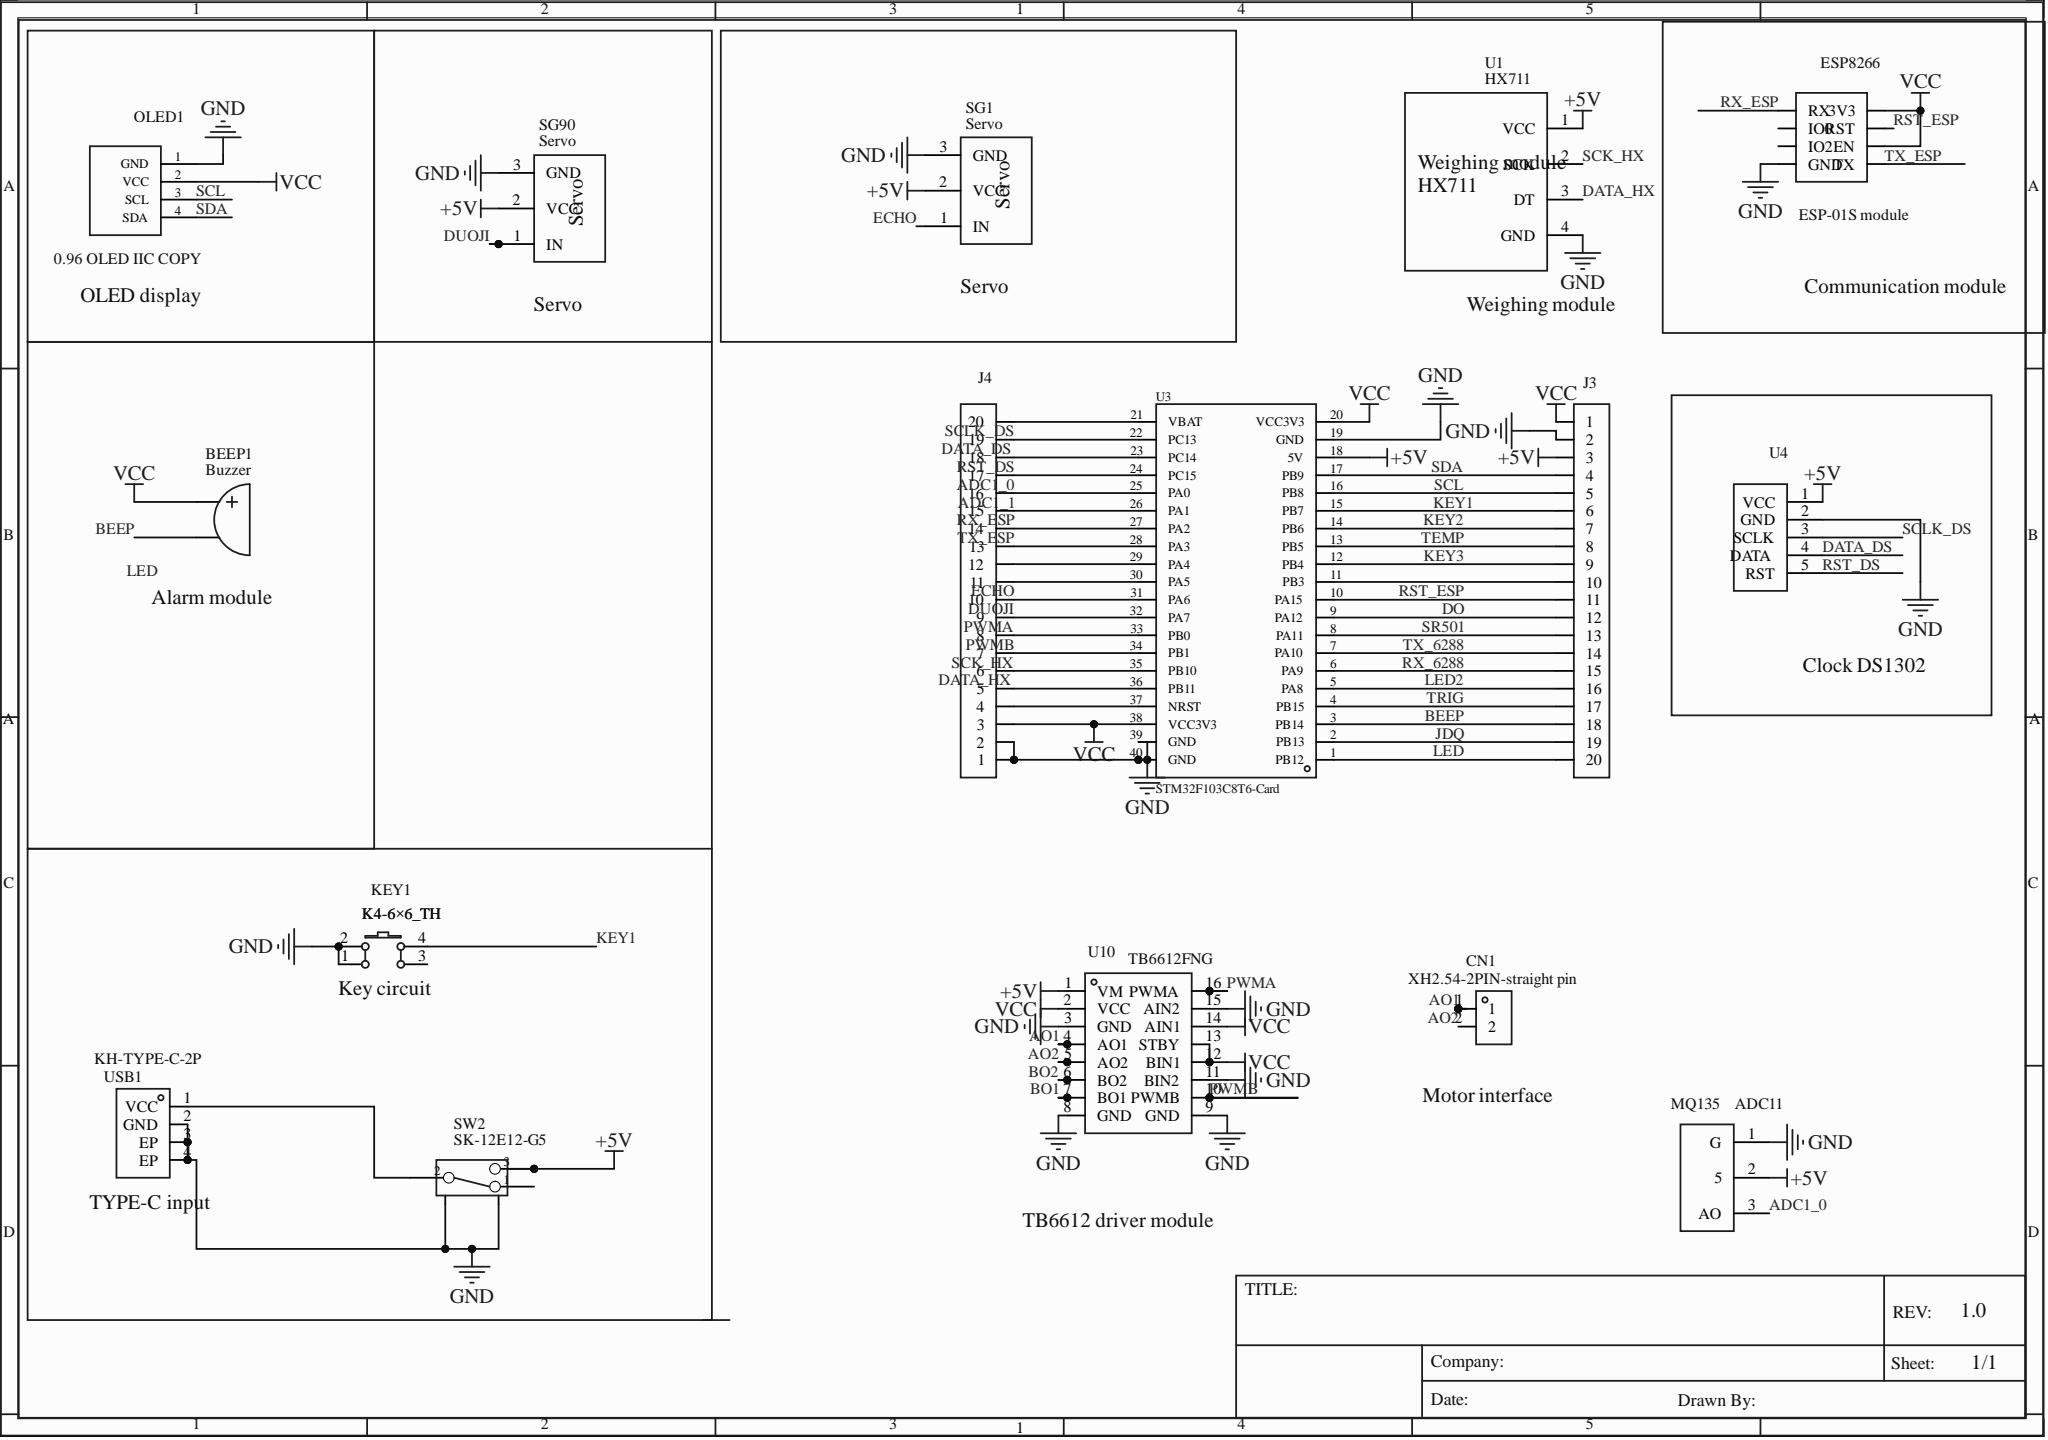Circuit board | Altium Designer | 16 parts | 40 nets
Bill of materials:
Comment,Description,Designator,Footprint,LibRef,Quantity
"MQ135","","ADC11","HDR-TH_3P-P2.54-V-F","MQ135","1"
"Buzzer","","BEEP1","BUZ-TH_BD11.8-P7.60_XHXDZ-TMB12065","蜂鸣器","1"
"XH2.54-2PIN-straight pin","","CN1","CONN-TH_XH2.54-2P","XH2.54-2PIN-直针","1"
"ESP-01S module","","ESP8266","WIFIM-TH_ESP-01S","ESP-01S模块","1"
"HDR-M-2.54_1x20","","J3, J4","HDR-M-2.54_1X20","HDR-M-2.54_1x20","2"
"K4-6×6_TH","","KEY1","KEY-TH_4P-L6.0-W6.0-P4.50-LS6.5","K2-1102DP-E4SW-04","1"
"0.96 OLED IIC COPY","","OLED1","OLED-TH_4P-L23.44-W19.0_ER-OLEDM0.66-1W-I2C","0.96 OLED IIC COPY","1"
"Servo","","SG1, SG90","HDR-TH_3P-P2.54-V-F","舵机","2"
"SK-12E12-G5","","SW2","SW-TH_SK-12E12-G5","SK-12E12-G5","1"
"HX711","","U1","HDR-TH_4P-P2.54-V-F","HX711","1"
"STM32F103C8T6-Card","","U3","CONN-TH_L53.3-W22.9_STM32F103C8T6-CARD","STM32F103C8T6-Card","1"
"Clock DS1302","","U4","HDR-TH_5P-P2.54-V-F","时钟DS1302","1"
"TB6612FNG","","U10","tb6612","TB6612FNG","1"
"KH-TYPE-C-2P","","USB1","USB-SMD_KH-TYPE-C-2P","KH-TYPE-C-2P","1"
Netlist (Protel format):
[
ADC11
HDR-TH_3P-P2.54-V-F
MQ135



]
[
BEEP1
BUZ-TH_BD11.8-P7.60_XHXDZ-TMB12065
Buzzer



]
[
CN1
CONN-TH_XH2.54-2P
XH2.54-2PIN-straight pin



]
[
ESP8266
WIFIM-TH_ESP-01S
ESP-01S module



]
[
J3
HDR-M-2.54_1X20
HDR-M-2.54_1x20



]
[
J4
HDR-M-2.54_1X20
HDR-M-2.54_1x20



]
[
KEY1
KEY-TH_4P-L6.0-W6.0-P4.50-LS6.5
K4-6×6_TH



]
[
OLED1
OLED-TH_4P-L23.44-W19.0_ER-OLEDM0.66-1W-I2C
0.96 OLED IIC COPY



]
[
SG1
HDR-TH_3P-P2.54-V-F
Servo



]
[
SG90
HDR-TH_3P-P2.54-V-F
Servo



]
[
SW2
SW-TH_SK-12E12-G5
SK-12E12-G5



]
[
U1
HDR-TH_4P-P2.54-V-F
HX711



]
[
U3
CONN-TH_L53.3-W22.9_STM32F103C8T6-CARD
STM32F103C8T6-Card



]
[
U4
HDR-TH_5P-P2.54-V-F
Clock DS1302



]
[
U10
tb6612
TB6612FNG



]
[
USB1
USB-SMD_KH-TYPE-C-2P
KH-TYPE-C-2P



]
(
VCC
BEEP1-1
ESP8266-1
ESP8266-3
J3-1
J4-3
OLED1-2
U3-20
U3-38
U10-2
U10-12
U10-13
U10-14
)
(
TX_ESP
ESP8266-4
J4-13
U3-28
)
(
TX_6288
J3-14
U3-7
)
(
TRIG
J3-17
U3-4
)
(
TEMP
J3-8
U3-13
)
(
SR501
J3-13
U3-8
)
(
SDA
J3-4
OLED1-4
U3-17
)
(
SCLK_DS
J4-19
U3-22
U4-3
)
(
SCL
J3-5
OLED1-3
U3-16
)
(
SCK_HX
J4-6
U1-2
U3-35
)
(
RX_ESP
ESP8266-8
J4-14
U3-27
)
(
RX_6288
J3-15
U3-6
)
(
RST_ESP
ESP8266-2
J3-11
U3-10
)
(
RST_DS
J4-17
U3-24
U4-5
)
(
PWMB
J4-7
U3-34
U10-10
)
(
PWMA
J4-8
U3-33
U10-16
)
(
NetSW2_2
SW2-2
USB1-1
)
(
NetJ4_20
J4-20
U3-21
)
(
NetJ4_12
J4-12
U3-29
)
(
NetJ4_11
J4-11
U3-30
)
(
NetJ4_4
J4-4
U3-37
)
(
NetJ3_10
J3-10
U3-11
)
(
LED2
J3-16
U3-5
)
(
LED
J3-20
U3-1
)
(
KEY3
J3-9
U3-12
)
(
KEY2
J3-7
U3-14
)
(
KEY1
J3-6
KEY1-4
U3-15
)
(
JDQ
J3-19
U3-2
)
(
GND
ADC11-1
ESP8266-5
J3-2
J4-1
J4-2
KEY1-1
KEY1-2
OLED1-1
SG1-3
SG90-3
SW2-4
SW2-5
U1-4
U3-19
U3-39
U3-40
U4-2
U10-3
U10-8
U10-9
U10-11
U10-15
USB1-2
USB1-3
USB1-4
)
(
ECHO
J4-10
SG1-1
U3-31
)
(
DUOJI
J4-9
SG90-1
U3-32
)
(
DO
J3-12
U3-9
)
(
DATA_HX
J4-5
U1-3
U3-36
)
(
DATA_DS
J4-18
U3-23
U4-4
)
(
BEEP
BEEP1-2
J3-18
U3-3
)
(
AO2
CN1-2
U10-5
)
(
AO1
CN1-1
U10-4
)
(
ADC1_1
J4-15
U3-26
)
(
ADC1_0
ADC11-3
J4-16
U3-25
)
(
+5V
ADC11-2
J3-3
SG1-2
SG90-2
SW2-3
U1-1
U3-18
U4-1
U10-1
)